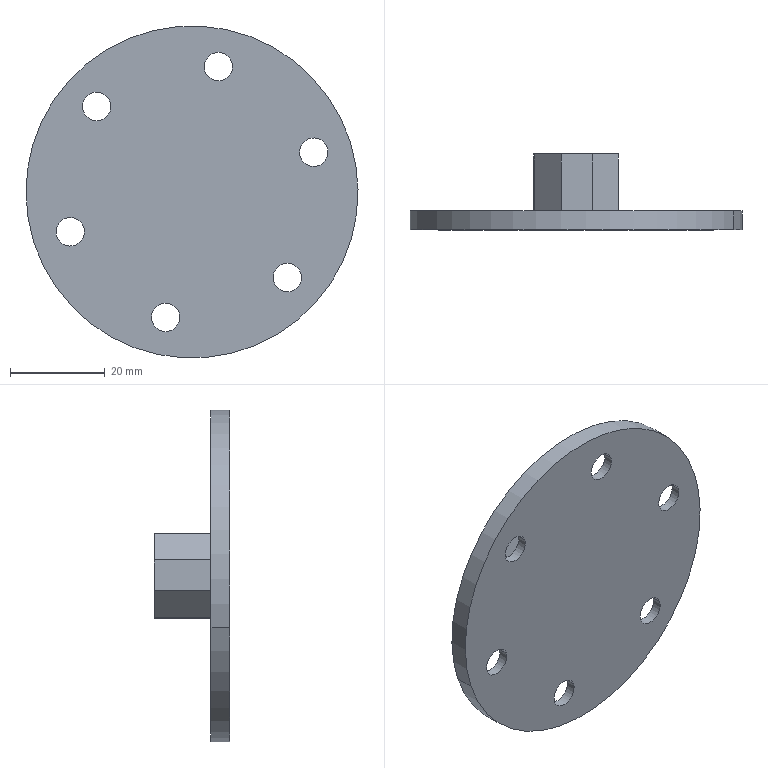Part | NX | features BREP 1 | 1 solid | 61 faces | box 70 x 16 x 70 mm | volume 15436 mm3 | cylinder 35 | plane 26 | commonest cylinder face diameters 6 x12 12 x12 4.2 x9 70 x2